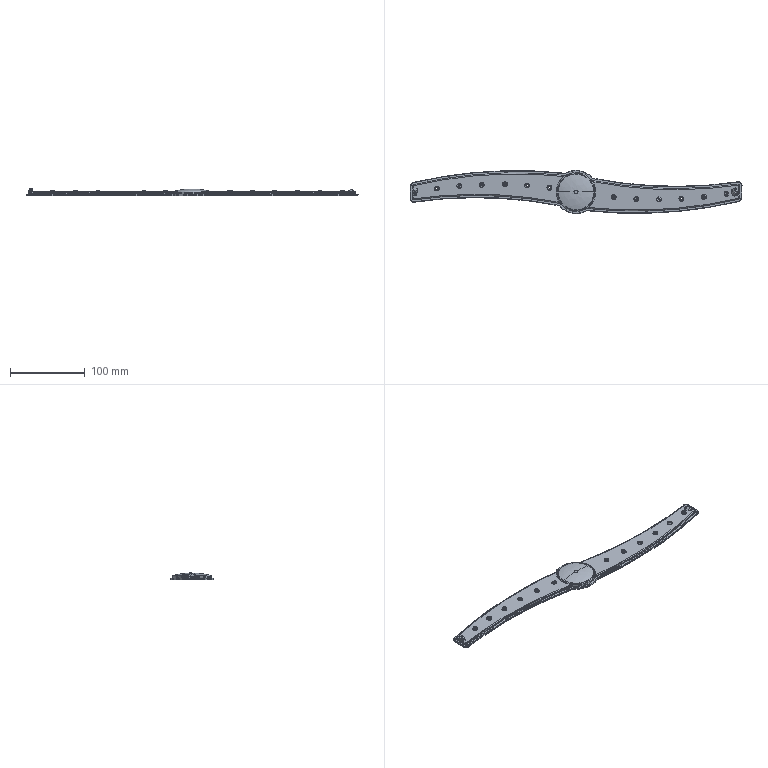Part | STEP file | ZXW722-L-15 | 1 solid | 372 faces | box 443.493 x 58 x 9.556 mm | volume 31671 mm3 | cylinder 155 | torus 87 | spline 83 | plane 45 | sphere 2 | commonest cylinder face diameters 3 x29 6 x29 2 x15 1 x14 9 x8 10 x8